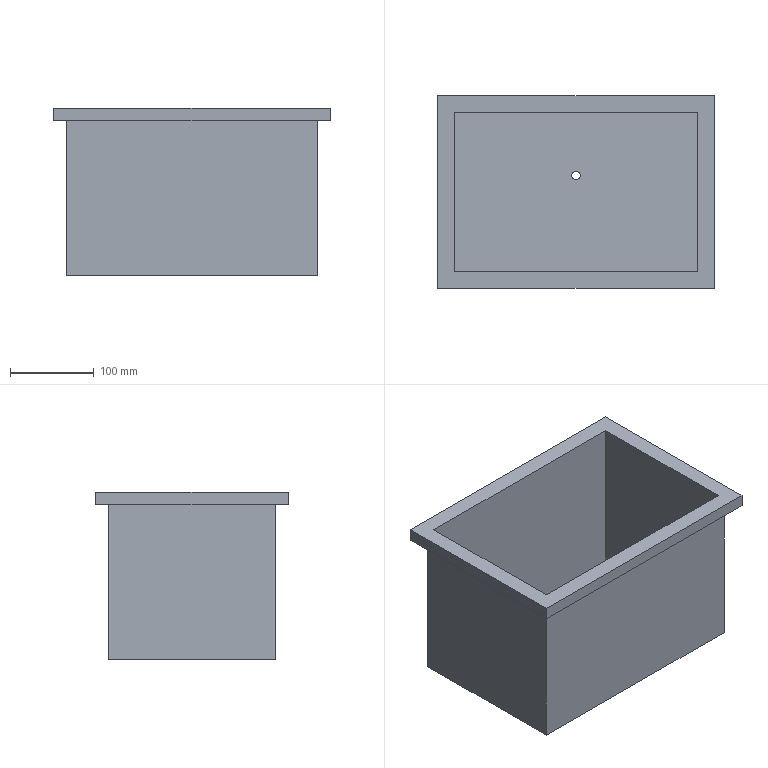Part | STEP file | Material box - copy | 1 solid | 18 faces | box 330 x 230 x 200 mm | volume 1493607 mm3 | plane 16 | cylinder 2 | commonest cylinder face diameters 10 x2
STEP:
#1=CARTESIAN_POINT('',(0.,0.,0.));
#2=DIRECTION('',(0.,0.,1.));
#3=DIRECTION('',(1.,0.,0.));
#4=AXIS2_PLACEMENT_3D('',#1,#2,#3);
#5=CARTESIAN_POINT('',(5.,20.,0.));
#6=VERTEX_POINT('',#5);
#7=CARTESIAN_POINT('',(5.,20.,5.));
#8=VERTEX_POINT('',#7);
#9=CARTESIAN_POINT('',(5.,20.,-5.));
#10=DIRECTION('',(0.,0.,1.));
#11=VECTOR('',#10,1.);
#12=LINE('',#9,#11);
#13=CARTESIAN_POINT('',(0.,20.,-5.));
#14=DIRECTION('',(0.,0.,1.));
#15=DIRECTION('',(1.,0.,0.));
#16=AXIS2_PLACEMENT_3D('',#13,#14,#15);
#17=CYLINDRICAL_SURFACE('',#16,5.);
#18=CARTESIAN_POINT('',(6.283,0.));
#19=DIRECTION('',(0.,1.));
#20=VECTOR('',#19,1.);
#21=LINE('',#18,#20);
#22=(GEOMETRIC_REPRESENTATION_CONTEXT(2)PARAMETRIC_REPRESENTATION_CONTEXT()REPRESENTATION_CONTEXT('',''));
#23=DEFINITIONAL_REPRESENTATION('',(#21),#22);
#24=PCURVE('',#17,#23);
#25=CARTESIAN_POINT('',(0.,20.,-5.));
#26=DIRECTION('',(0.,0.,1.));
#27=DIRECTION('',(1.,0.,0.));
#28=AXIS2_PLACEMENT_3D('',#25,#26,#27);
#29=CYLINDRICAL_SURFACE('',#28,5.);
#30=CARTESIAN_POINT('',(0.,0.));
#31=DIRECTION('',(0.,1.));
#32=VECTOR('',#31,1.);
#33=LINE('',#30,#32);
#34=(GEOMETRIC_REPRESENTATION_CONTEXT(2)PARAMETRIC_REPRESENTATION_CONTEXT()REPRESENTATION_CONTEXT('',''));
#35=DEFINITIONAL_REPRESENTATION('',(#33),#34);
#36=PCURVE('',#29,#35);
#37=SURFACE_CURVE('',#12,(#24,#36),.PCURVE_S1.);
#38=EDGE_CURVE('',#6,#8,#37,.T.);
#39=ORIENTED_EDGE('',*,*,#38,.T.);
#40=CARTESIAN_POINT('',(-5.,20.,5.));
#41=VERTEX_POINT('',#40);
#42=CARTESIAN_POINT('',(0.,20.,5.));
#43=DIRECTION('',(0.,0.,-1.));
#44=DIRECTION('',(1.,0.,0.));
#45=AXIS2_PLACEMENT_3D('',#42,#43,#44);
#46=CIRCLE('',#45,5.);
#47=CARTESIAN_POINT('',(6.283,10.));
#48=DIRECTION('',(-1.,0.));
#49=VECTOR('',#48,1.);
#50=LINE('',#47,#49);
#51=(GEOMETRIC_REPRESENTATION_CONTEXT(2)PARAMETRIC_REPRESENTATION_CONTEXT()REPRESENTATION_CONTEXT('',''));
#52=DEFINITIONAL_REPRESENTATION('',(#50),#51);
#53=PCURVE('',#17,#52);
#54=CARTESIAN_POINT('',(0.,0.,5.));
#55=DIRECTION('',(0.,0.,1.));
#56=DIRECTION('',(1.,0.,0.));
#57=AXIS2_PLACEMENT_3D('',#54,#55,#56);
#58=PLANE('',#57);
#59=CARTESIAN_POINT('',(5.,20.));
#60=CARTESIAN_POINT('',(5.,11.34));
#61=CARTESIAN_POINT('',(-2.5,15.67));
#62=CARTESIAN_POINT('',(-10.,20.));
#63=CARTESIAN_POINT('',(-2.5,24.33));
#64=CARTESIAN_POINT('',(5.,28.66));
#65=CARTESIAN_POINT('',(5.,20.));
#66=(BOUNDED_CURVE()B_SPLINE_CURVE(2,(#59,#60,#61,#62,#63,#64,#65),.UNSPECIFIED.,.T.,.F.)B_SPLINE_CURVE_WITH_KNOTS((1,2,2,2,2,1),(-2.094,0.,2.094,4.189,6.283,8.378),.UNSPECIFIED.)CURVE()GEOMETRIC_REPRESENTATION_ITEM()RATIONAL_B_SPLINE_CURVE((1.,0.5,1.,0.5,1.,0.5,1.))REPRESENTATION_ITEM(''));
#67=(GEOMETRIC_REPRESENTATION_CONTEXT(2)PARAMETRIC_REPRESENTATION_CONTEXT()REPRESENTATION_CONTEXT('',''));
#68=DEFINITIONAL_REPRESENTATION('',(#66),#67);
#69=PCURVE('',#58,#68);
#70=SURFACE_CURVE('',#46,(#53,#69),.PCURVE_S1.);
#71=EDGE_CURVE('',#8,#41,#70,.T.);
#72=ORIENTED_EDGE('',*,*,#71,.T.);
#73=CARTESIAN_POINT('',(-5.,20.,0.));
#74=VERTEX_POINT('',#73);
#75=CARTESIAN_POINT('',(-5.,20.,-5.));
#76=DIRECTION('',(0.,0.,1.));
#77=VECTOR('',#76,1.);
#78=LINE('',#75,#77);
#79=CARTESIAN_POINT('',(3.142,0.));
#80=DIRECTION('',(0.,1.));
#81=VECTOR('',#80,1.);
#82=LINE('',#79,#81);
#83=(GEOMETRIC_REPRESENTATION_CONTEXT(2)PARAMETRIC_REPRESENTATION_CONTEXT()REPRESENTATION_CONTEXT('',''));
#84=DEFINITIONAL_REPRESENTATION('',(#82),#83);
#85=PCURVE('',#17,#84);
#86=CARTESIAN_POINT('',(3.142,0.));
#87=DIRECTION('',(0.,1.));
#88=VECTOR('',#87,1.);
#89=LINE('',#86,#88);
#90=(GEOMETRIC_REPRESENTATION_CONTEXT(2)PARAMETRIC_REPRESENTATION_CONTEXT()REPRESENTATION_CONTEXT('',''));
#91=DEFINITIONAL_REPRESENTATION('',(#89),#90);
#92=PCURVE('',#29,#91);
#93=SURFACE_CURVE('',#78,(#85,#92),.PCURVE_S1.);
#94=EDGE_CURVE('',#74,#41,#93,.T.);
#95=ORIENTED_EDGE('',*,*,#94,.F.);
#96=CARTESIAN_POINT('',(0.,20.,0.));
#97=DIRECTION('',(0.,0.,-1.));
#98=DIRECTION('',(1.,0.,0.));
#99=AXIS2_PLACEMENT_3D('',#96,#97,#98);
#100=CIRCLE('',#99,5.);
#101=CARTESIAN_POINT('',(6.283,5.));
#102=DIRECTION('',(-1.,0.));
#103=VECTOR('',#102,1.);
#104=LINE('',#101,#103);
#105=(GEOMETRIC_REPRESENTATION_CONTEXT(2)PARAMETRIC_REPRESENTATION_CONTEXT()REPRESENTATION_CONTEXT('',''));
#106=DEFINITIONAL_REPRESENTATION('',(#104),#105);
#107=PCURVE('',#17,#106);
#108=CARTESIAN_POINT('',(0.,0.,0.));
#109=DIRECTION('',(0.,0.,1.));
#110=DIRECTION('',(1.,0.,0.));
#111=AXIS2_PLACEMENT_3D('',#108,#109,#110);
#112=PLANE('',#111);
#113=CARTESIAN_POINT('',(5.,20.));
#114=CARTESIAN_POINT('',(5.,11.34));
#115=CARTESIAN_POINT('',(-2.5,15.67));
#116=CARTESIAN_POINT('',(-10.,20.));
#117=CARTESIAN_POINT('',(-2.5,24.33));
#118=CARTESIAN_POINT('',(5.,28.66));
#119=CARTESIAN_POINT('',(5.,20.));
#120=(BOUNDED_CURVE()B_SPLINE_CURVE(2,(#113,#114,#115,#116,#117,#118,#119),.UNSPECIFIED.,.T.,.F.)B_SPLINE_CURVE_WITH_KNOTS((1,2,2,2,2,1),(-2.094,0.,2.094,4.189,6.283,8.378),.UNSPECIFIED.)CURVE()GEOMETRIC_REPRESENTATION_ITEM()RATIONAL_B_SPLINE_CURVE((1.,0.5,1.,0.5,1.,0.5,1.))REPRESENTATION_ITEM(''));
#121=(GEOMETRIC_REPRESENTATION_CONTEXT(2)PARAMETRIC_REPRESENTATION_CONTEXT()REPRESENTATION_CONTEXT('',''));
#122=DEFINITIONAL_REPRESENTATION('',(#120),#121);
#123=PCURVE('',#112,#122);
#124=SURFACE_CURVE('',#100,(#107,#123),.PCURVE_S1.);
#125=EDGE_CURVE('',#6,#74,#124,.T.);
#126=ORIENTED_EDGE('',*,*,#125,.F.);
#127=EDGE_LOOP('',(#39,#72,#95,#126));
#128=FACE_BOUND('',#127,.F.);
#129=ADVANCED_FACE('',(#128),#17,.F.);
#130=CARTESIAN_POINT('',(-150.,-100.,0.));
#131=VERTEX_POINT('',#130);
#132=CARTESIAN_POINT('',(150.,-100.,0.));
#133=VERTEX_POINT('',#132);
#134=CARTESIAN_POINT('',(0.,-100.,0.));
#135=DIRECTION('',(1.,0.,0.));
#136=VECTOR('',#135,1.);
#137=LINE('',#134,#136);
#138=CARTESIAN_POINT('',(0.,-100.));
#139=DIRECTION('',(1.,0.));
#140=VECTOR('',#139,1.);
#141=LINE('',#138,#140);
#142=(GEOMETRIC_REPRESENTATION_CONTEXT(2)PARAMETRIC_REPRESENTATION_CONTEXT()REPRESENTATION_CONTEXT('',''));
#143=DEFINITIONAL_REPRESENTATION('',(#141),#142);
#144=PCURVE('',#112,#143);
#145=CARTESIAN_POINT('',(-150.,-100.,200.));
#146=DIRECTION('',(0.,1.,0.));
#147=DIRECTION('',(0.,0.,1.));
#148=AXIS2_PLACEMENT_3D('',#145,#146,#147);
#149=PLANE('',#148);
#150=CARTESIAN_POINT('',(-200.,150.));
#151=DIRECTION('',(0.,1.));
#152=VECTOR('',#151,1.);
#153=LINE('',#150,#152);
#154=(GEOMETRIC_REPRESENTATION_CONTEXT(2)PARAMETRIC_REPRESENTATION_CONTEXT()REPRESENTATION_CONTEXT('',''));
#155=DEFINITIONAL_REPRESENTATION('',(#153),#154);
#156=PCURVE('',#149,#155);
#157=SURFACE_CURVE('',#137,(#144,#156),.PCURVE_S1.);
#158=EDGE_CURVE('',#131,#133,#157,.T.);
#159=ORIENTED_EDGE('',*,*,#158,.F.);
#160=CARTESIAN_POINT('',(-150.,100.,0.));
#161=VERTEX_POINT('',#160);
#162=CARTESIAN_POINT('',(-150.,0.,0.));
#163=DIRECTION('',(0.,-1.,0.));
#164=VECTOR('',#163,1.);
#165=LINE('',#162,#164);
#166=CARTESIAN_POINT('',(-150.,0.));
#167=DIRECTION('',(0.,-1.));
#168=VECTOR('',#167,1.);
#169=LINE('',#166,#168);
#170=(GEOMETRIC_REPRESENTATION_CONTEXT(2)PARAMETRIC_REPRESENTATION_CONTEXT()REPRESENTATION_CONTEXT('',''));
#171=DEFINITIONAL_REPRESENTATION('',(#169),#170);
#172=PCURVE('',#112,#171);
#173=CARTESIAN_POINT('',(-150.,100.,200.));
#174=DIRECTION('',(1.,0.,0.));
#175=DIRECTION('',(0.,0.,-1.));
#176=AXIS2_PLACEMENT_3D('',#173,#174,#175);
#177=PLANE('',#176);
#178=CARTESIAN_POINT('',(200.,-100.));
#179=DIRECTION('',(0.,-1.));
#180=VECTOR('',#179,1.);
#181=LINE('',#178,#180);
#182=(GEOMETRIC_REPRESENTATION_CONTEXT(2)PARAMETRIC_REPRESENTATION_CONTEXT()REPRESENTATION_CONTEXT('',''));
#183=DEFINITIONAL_REPRESENTATION('',(#181),#182);
#184=PCURVE('',#177,#183);
#185=SURFACE_CURVE('',#165,(#172,#184),.PCURVE_S1.);
#186=EDGE_CURVE('',#161,#131,#185,.T.);
#187=ORIENTED_EDGE('',*,*,#186,.F.);
#188=CARTESIAN_POINT('',(150.,100.,0.));
#189=VERTEX_POINT('',#188);
#190=CARTESIAN_POINT('',(0.,100.,0.));
#191=DIRECTION('',(-1.,0.,0.));
#192=VECTOR('',#191,1.);
#193=LINE('',#190,#192);
#194=CARTESIAN_POINT('',(0.,100.));
#195=DIRECTION('',(-1.,0.));
#196=VECTOR('',#195,1.);
#197=LINE('',#194,#196);
#198=(GEOMETRIC_REPRESENTATION_CONTEXT(2)PARAMETRIC_REPRESENTATION_CONTEXT()REPRESENTATION_CONTEXT('',''));
#199=DEFINITIONAL_REPRESENTATION('',(#197),#198);
#200=PCURVE('',#112,#199);
#201=CARTESIAN_POINT('',(-150.,100.,200.));
#202=DIRECTION('',(0.,-1.,0.));
#203=DIRECTION('',(0.,0.,-1.));
#204=AXIS2_PLACEMENT_3D('',#201,#202,#203);
#205=PLANE('',#204);
#206=CARTESIAN_POINT('',(200.,150.));
#207=DIRECTION('',(0.,-1.));
#208=VECTOR('',#207,1.);
#209=LINE('',#206,#208);
#210=(GEOMETRIC_REPRESENTATION_CONTEXT(2)PARAMETRIC_REPRESENTATION_CONTEXT()REPRESENTATION_CONTEXT('',''));
#211=DEFINITIONAL_REPRESENTATION('',(#209),#210);
#212=PCURVE('',#205,#211);
#213=SURFACE_CURVE('',#193,(#200,#212),.PCURVE_S1.);
#214=EDGE_CURVE('',#189,#161,#213,.T.);
#215=ORIENTED_EDGE('',*,*,#214,.F.);
#216=CARTESIAN_POINT('',(150.,0.,0.));
#217=DIRECTION('',(0.,1.,0.));
#218=VECTOR('',#217,1.);
#219=LINE('',#216,#218);
#220=CARTESIAN_POINT('',(150.,0.));
#221=DIRECTION('',(0.,1.));
#222=VECTOR('',#221,1.);
#223=LINE('',#220,#222);
#224=(GEOMETRIC_REPRESENTATION_CONTEXT(2)PARAMETRIC_REPRESENTATION_CONTEXT()REPRESENTATION_CONTEXT('',''));
#225=DEFINITIONAL_REPRESENTATION('',(#223),#224);
#226=PCURVE('',#112,#225);
#227=CARTESIAN_POINT('',(150.,100.,200.));
#228=DIRECTION('',(-1.,0.,0.));
#229=DIRECTION('',(0.,0.,1.));
#230=AXIS2_PLACEMENT_3D('',#227,#228,#229);
#231=PLANE('',#230);
#232=CARTESIAN_POINT('',(-200.,-100.));
#233=DIRECTION('',(0.,1.));
#234=VECTOR('',#233,1.);
#235=LINE('',#232,#234);
#236=(GEOMETRIC_REPRESENTATION_CONTEXT(2)PARAMETRIC_REPRESENTATION_CONTEXT()REPRESENTATION_CONTEXT('',''));
#237=DEFINITIONAL_REPRESENTATION('',(#235),#236);
#238=PCURVE('',#231,#237);
#239=SURFACE_CURVE('',#219,(#226,#238),.PCURVE_S1.);
#240=EDGE_CURVE('',#133,#189,#239,.T.);
#241=ORIENTED_EDGE('',*,*,#240,.F.);
#242=EDGE_LOOP('',(#159,#187,#215,#241));
#243=FACE_BOUND('',#242,.T.);
#244=ORIENTED_EDGE('',*,*,#125,.F.);
#245=CARTESIAN_POINT('',(0.,20.,0.));
#246=DIRECTION('',(0.,0.,-1.));
#247=DIRECTION('',(1.,0.,0.));
#248=AXIS2_PLACEMENT_3D('',#245,#246,#247);
#249=CIRCLE('',#248,5.);
#250=CARTESIAN_POINT('',(5.,20.));
#251=CARTESIAN_POINT('',(5.,11.34));
#252=CARTESIAN_POINT('',(-2.5,15.67));
#253=CARTESIAN_POINT('',(-10.,20.));
#254=CARTESIAN_POINT('',(-2.5,24.33));
#255=CARTESIAN_POINT('',(5.,28.66));
#256=CARTESIAN_POINT('',(5.,20.));
#257=(BOUNDED_CURVE()B_SPLINE_CURVE(2,(#250,#251,#252,#253,#254,#255,#256),.UNSPECIFIED.,.T.,.F.)B_SPLINE_CURVE_WITH_KNOTS((1,2,2,2,2,1),(-2.094,0.,2.094,4.189,6.283,8.378),.UNSPECIFIED.)CURVE()GEOMETRIC_REPRESENTATION_ITEM()RATIONAL_B_SPLINE_CURVE((1.,0.5,1.,0.5,1.,0.5,1.))REPRESENTATION_ITEM(''));
#258=(GEOMETRIC_REPRESENTATION_CONTEXT(2)PARAMETRIC_REPRESENTATION_CONTEXT()REPRESENTATION_CONTEXT('',''));
#259=DEFINITIONAL_REPRESENTATION('',(#257),#258);
#260=PCURVE('',#112,#259);
#261=CARTESIAN_POINT('',(6.283,5.));
#262=DIRECTION('',(-1.,0.));
#263=VECTOR('',#262,1.);
#264=LINE('',#261,#263);
#265=(GEOMETRIC_REPRESENTATION_CONTEXT(2)PARAMETRIC_REPRESENTATION_CONTEXT()REPRESENTATION_CONTEXT('',''));
#266=DEFINITIONAL_REPRESENTATION('',(#264),#265);
#267=PCURVE('',#29,#266);
#268=SURFACE_CURVE('',#249,(#260,#267),.PCURVE_S1.);
#269=EDGE_CURVE('',#74,#6,#268,.T.);
#270=ORIENTED_EDGE('',*,*,#269,.F.);
#271=EDGE_LOOP('',(#244,#270));
#272=FACE_BOUND('',#271,.T.);
#273=ADVANCED_FACE('',(#243,#272),#112,.F.);
#274=CARTESIAN_POINT('',(150.,-100.,185.));
#275=VERTEX_POINT('',#274);
#276=CARTESIAN_POINT('',(150.,100.,185.));
#277=VERTEX_POINT('',#276);
#278=CARTESIAN_POINT('',(150.,100.,185.));
#279=DIRECTION('',(0.,1.,0.));
#280=VECTOR('',#279,1.);
#281=LINE('',#278,#280);
#282=CARTESIAN_POINT('',(-15.,0.));
#283=DIRECTION('',(0.,1.));
#284=VECTOR('',#283,1.);
#285=LINE('',#282,#284);
#286=(GEOMETRIC_REPRESENTATION_CONTEXT(2)PARAMETRIC_REPRESENTATION_CONTEXT()REPRESENTATION_CONTEXT('',''));
#287=DEFINITIONAL_REPRESENTATION('',(#285),#286);
#288=PCURVE('',#231,#287);
#289=CARTESIAN_POINT('',(0.,0.,185.));
#290=DIRECTION('',(0.,0.,-1.));
#291=DIRECTION('',(-1.,0.,0.));
#292=AXIS2_PLACEMENT_3D('',#289,#290,#291);
#293=PLANE('',#292);
#294=CARTESIAN_POINT('',(-150.,100.));
#295=DIRECTION('',(0.,1.));
#296=VECTOR('',#295,1.);
#297=LINE('',#294,#296);
#298=(GEOMETRIC_REPRESENTATION_CONTEXT(2)PARAMETRIC_REPRESENTATION_CONTEXT()REPRESENTATION_CONTEXT('',''));
#299=DEFINITIONAL_REPRESENTATION('',(#297),#298);
#300=PCURVE('',#293,#299);
#301=SURFACE_CURVE('',#281,(#288,#300),.PCURVE_S1.);
#302=EDGE_CURVE('',#275,#277,#301,.T.);
#303=ORIENTED_EDGE('',*,*,#302,.F.);
#304=CARTESIAN_POINT('',(150.,-100.,200.));
#305=DIRECTION('',(0.,0.,1.));
#306=VECTOR('',#305,1.);
#307=LINE('',#304,#306);
#308=CARTESIAN_POINT('',(0.,-200.));
#309=DIRECTION('',(1.,0.));
#310=VECTOR('',#309,1.);
#311=LINE('',#308,#310);
#312=(GEOMETRIC_REPRESENTATION_CONTEXT(2)PARAMETRIC_REPRESENTATION_CONTEXT()REPRESENTATION_CONTEXT('',''));
#313=DEFINITIONAL_REPRESENTATION('',(#311),#312);
#314=PCURVE('',#231,#313);
#315=CARTESIAN_POINT('',(0.,300.));
#316=DIRECTION('',(1.,0.));
#317=VECTOR('',#316,1.);
#318=LINE('',#315,#317);
#319=(GEOMETRIC_REPRESENTATION_CONTEXT(2)PARAMETRIC_REPRESENTATION_CONTEXT()REPRESENTATION_CONTEXT('',''));
#320=DEFINITIONAL_REPRESENTATION('',(#318),#319);
#321=PCURVE('',#149,#320);
#322=SURFACE_CURVE('',#307,(#314,#321),.PCURVE_S1.);
#323=EDGE_CURVE('',#133,#275,#322,.T.);
#324=ORIENTED_EDGE('',*,*,#323,.F.);
#325=ORIENTED_EDGE('',*,*,#240,.T.);
#326=CARTESIAN_POINT('',(150.,100.,200.));
#327=DIRECTION('',(0.,0.,-1.));
#328=VECTOR('',#327,1.);
#329=LINE('',#326,#328);
#330=CARTESIAN_POINT('',(0.,0.));
#331=DIRECTION('',(-1.,0.));
#332=VECTOR('',#331,1.);
#333=LINE('',#330,#332);
#334=(GEOMETRIC_REPRESENTATION_CONTEXT(2)PARAMETRIC_REPRESENTATION_CONTEXT()REPRESENTATION_CONTEXT('',''));
#335=DEFINITIONAL_REPRESENTATION('',(#333),#334);
#336=PCURVE('',#231,#335);
#337=CARTESIAN_POINT('',(0.,300.));
#338=DIRECTION('',(1.,0.));
#339=VECTOR('',#338,1.);
#340=LINE('',#337,#339);
#341=(GEOMETRIC_REPRESENTATION_CONTEXT(2)PARAMETRIC_REPRESENTATION_CONTEXT()REPRESENTATION_CONTEXT('',''));
#342=DEFINITIONAL_REPRESENTATION('',(#340),#341);
#343=PCURVE('',#205,#342);
#344=SURFACE_CURVE('',#329,(#336,#343),.PCURVE_S1.);
#345=EDGE_CURVE('',#277,#189,#344,.T.);
#346=ORIENTED_EDGE('',*,*,#345,.F.);
#347=EDGE_LOOP('',(#303,#324,#325,#346));
#348=FACE_BOUND('',#347,.T.);
#349=ADVANCED_FACE('',(#348),#231,.F.);
#350=CARTESIAN_POINT('',(-150.,-100.,185.));
#351=VERTEX_POINT('',#350);
#352=CARTESIAN_POINT('',(-150.,-100.,185.));
#353=DIRECTION('',(1.,0.,0.));
#354=VECTOR('',#353,1.);
#355=LINE('',#352,#354);
#356=CARTESIAN_POINT('',(-15.,0.));
#357=DIRECTION('',(0.,1.));
#358=VECTOR('',#357,1.);
#359=LINE('',#356,#358);
#360=(GEOMETRIC_REPRESENTATION_CONTEXT(2)PARAMETRIC_REPRESENTATION_CONTEXT()REPRESENTATION_CONTEXT('',''));
#361=DEFINITIONAL_REPRESENTATION('',(#359),#360);
#362=PCURVE('',#149,#361);
#363=CARTESIAN_POINT('',(150.,-100.));
#364=DIRECTION('',(-1.,0.));
#365=VECTOR('',#364,1.);
#366=LINE('',#363,#365);
#367=(GEOMETRIC_REPRESENTATION_CONTEXT(2)PARAMETRIC_REPRESENTATION_CONTEXT()REPRESENTATION_CONTEXT('',''));
#368=DEFINITIONAL_REPRESENTATION('',(#366),#367);
#369=PCURVE('',#293,#368);
#370=SURFACE_CURVE('',#355,(#362,#369),.PCURVE_S1.);
#371=EDGE_CURVE('',#351,#275,#370,.T.);
#372=ORIENTED_EDGE('',*,*,#371,.F.);
#373=CARTESIAN_POINT('',(-150.,-100.,200.));
#374=DIRECTION('',(0.,0.,1.));
#375=VECTOR('',#374,1.);
#376=LINE('',#373,#375);
#377=CARTESIAN_POINT('',(0.,0.));
#378=DIRECTION('',(1.,0.));
#379=VECTOR('',#378,1.);
#380=LINE('',#377,#379);
#381=(GEOMETRIC_REPRESENTATION_CONTEXT(2)PARAMETRIC_REPRESENTATION_CONTEXT()REPRESENTATION_CONTEXT('',''));
#382=DEFINITIONAL_REPRESENTATION('',(#380),#381);
#383=PCURVE('',#149,#382);
#384=CARTESIAN_POINT('',(0.,-200.));
#385=DIRECTION('',(-1.,0.));
#386=VECTOR('',#385,1.);
#387=LINE('',#384,#386);
#388=(GEOMETRIC_REPRESENTATION_CONTEXT(2)PARAMETRIC_REPRESENTATION_CONTEXT()REPRESENTATION_CONTEXT('',''));
#389=DEFINITIONAL_REPRESENTATION('',(#387),#388);
#390=PCURVE('',#177,#389);
#391=SURFACE_CURVE('',#376,(#383,#390),.PCURVE_S1.);
#392=EDGE_CURVE('',#131,#351,#391,.T.);
#393=ORIENTED_EDGE('',*,*,#392,.F.);
#394=ORIENTED_EDGE('',*,*,#158,.T.);
#395=ORIENTED_EDGE('',*,*,#323,.T.);
#396=EDGE_LOOP('',(#372,#393,#394,#395));
#397=FACE_BOUND('',#396,.T.);
#398=ADVANCED_FACE('',(#397),#149,.F.);
#399=CARTESIAN_POINT('',(-150.,100.,185.));
#400=VERTEX_POINT('',#399);
#401=CARTESIAN_POINT('',(-150.,100.,185.));
#402=DIRECTION('',(0.,-1.,0.));
#403=VECTOR('',#402,1.);
#404=LINE('',#401,#403);
#405=CARTESIAN_POINT('',(15.,0.));
#406=DIRECTION('',(0.,-1.));
#407=VECTOR('',#406,1.);
#408=LINE('',#405,#407);
#409=(GEOMETRIC_REPRESENTATION_CONTEXT(2)PARAMETRIC_REPRESENTATION_CONTEXT()REPRESENTATION_CONTEXT('',''));
#410=DEFINITIONAL_REPRESENTATION('',(#408),#409);
#411=PCURVE('',#177,#410);
#412=CARTESIAN_POINT('',(150.,100.));
#413=DIRECTION('',(0.,-1.));
#414=VECTOR('',#413,1.);
#415=LINE('',#412,#414);
#416=(GEOMETRIC_REPRESENTATION_CONTEXT(2)PARAMETRIC_REPRESENTATION_CONTEXT()REPRESENTATION_CONTEXT('',''));
#417=DEFINITIONAL_REPRESENTATION('',(#415),#416);
#418=PCURVE('',#293,#417);
#419=SURFACE_CURVE('',#404,(#411,#418),.PCURVE_S1.);
#420=EDGE_CURVE('',#400,#351,#419,.T.);
#421=ORIENTED_EDGE('',*,*,#420,.F.);
#422=CARTESIAN_POINT('',(-150.,100.,200.));
#423=DIRECTION('',(0.,0.,1.));
#424=VECTOR('',#423,1.);
#425=LINE('',#422,#424);
#426=CARTESIAN_POINT('',(0.,0.));
#427=DIRECTION('',(-1.,0.));
#428=VECTOR('',#427,1.);
#429=LINE('',#426,#428);
#430=(GEOMETRIC_REPRESENTATION_CONTEXT(2)PARAMETRIC_REPRESENTATION_CONTEXT()REPRESENTATION_CONTEXT('',''));
#431=DEFINITIONAL_REPRESENTATION('',(#429),#430);
#432=PCURVE('',#177,#431);
#433=CARTESIAN_POINT('',(0.,0.));
#434=DIRECTION('',(-1.,0.));
#435=VECTOR('',#434,1.);
#436=LINE('',#433,#435);
#437=(GEOMETRIC_REPRESENTATION_CONTEXT(2)PARAMETRIC_REPRESENTATION_CONTEXT()REPRESENTATION_CONTEXT('',''));
#438=DEFINITIONAL_REPRESENTATION('',(#436),#437);
#439=PCURVE('',#205,#438);
#440=SURFACE_CURVE('',#425,(#432,#439),.PCURVE_S1.);
#441=EDGE_CURVE('',#161,#400,#440,.T.);
#442=ORIENTED_EDGE('',*,*,#441,.F.);
#443=ORIENTED_EDGE('',*,*,#186,.T.);
#444=ORIENTED_EDGE('',*,*,#392,.T.);
#445=EDGE_LOOP('',(#421,#442,#443,#444));
#446=FACE_BOUND('',#445,.T.);
#447=ADVANCED_FACE('',(#446),#177,.F.);
#448=CARTESIAN_POINT('',(-150.,100.,185.));
#449=DIRECTION('',(-1.,0.,0.));
#450=VECTOR('',#449,1.);
#451=LINE('',#448,#450);
#452=CARTESIAN_POINT('',(15.,0.));
#453=DIRECTION('',(0.,-1.));
#454=VECTOR('',#453,1.);
#455=LINE('',#452,#454);
#456=(GEOMETRIC_REPRESENTATION_CONTEXT(2)PARAMETRIC_REPRESENTATION_CONTEXT()REPRESENTATION_CONTEXT('',''));
#457=DEFINITIONAL_REPRESENTATION('',(#455),#456);
#458=PCURVE('',#205,#457);
#459=CARTESIAN_POINT('',(150.,100.));
#460=DIRECTION('',(1.,0.));
#461=VECTOR('',#460,1.);
#462=LINE('',#459,#461);
#463=(GEOMETRIC_REPRESENTATION_CONTEXT(2)PARAMETRIC_REPRESENTATION_CONTEXT()REPRESENTATION_CONTEXT('',''));
#464=DEFINITIONAL_REPRESENTATION('',(#462),#463);
#465=PCURVE('',#293,#464);
#466=SURFACE_CURVE('',#451,(#458,#465),.PCURVE_S1.);
#467=EDGE_CURVE('',#277,#400,#466,.T.);
#468=ORIENTED_EDGE('',*,*,#467,.F.);
#469=ORIENTED_EDGE('',*,*,#345,.T.);
#470=ORIENTED_EDGE('',*,*,#214,.T.);
#471=ORIENTED_EDGE('',*,*,#441,.T.);
#472=EDGE_LOOP('',(#468,#469,#470,#471));
#473=FACE_BOUND('',#472,.T.);
#474=ADVANCED_FACE('',(#473),#205,.F.);
#475=CARTESIAN_POINT('',(0.,20.,5.));
#476=DIRECTION('',(0.,0.,-1.));
#477=DIRECTION('',(1.,0.,0.));
#478=AXIS2_PLACEMENT_3D('',#475,#476,#477);
#479=CIRCLE('',#478,5.);
#480=CARTESIAN_POINT('',(6.283,10.));
#481=DIRECTION('',(-1.,0.));
#482=VECTOR('',#481,1.);
#483=LINE('',#480,#482);
#484=(GEOMETRIC_REPRESENTATION_CONTEXT(2)PARAMETRIC_REPRESENTATION_CONTEXT()REPRESENTATION_CONTEXT('',''));
#485=DEFINITIONAL_REPRESENTATION('',(#483),#484);
#486=PCURVE('',#29,#485);
#487=CARTESIAN_POINT('',(5.,20.));
#488=CARTESIAN_POINT('',(5.,11.34));
#489=CARTESIAN_POINT('',(-2.5,15.67));
#490=CARTESIAN_POINT('',(-10.,20.));
#491=CARTESIAN_POINT('',(-2.5,24.33));
#492=CARTESIAN_POINT('',(5.,28.66));
#493=CARTESIAN_POINT('',(5.,20.));
#494=(BOUNDED_CURVE()B_SPLINE_CURVE(2,(#487,#488,#489,#490,#491,#492,#493),.UNSPECIFIED.,.T.,.F.)B_SPLINE_CURVE_WITH_KNOTS((1,2,2,2,2,1),(-2.094,0.,2.094,4.189,6.283,8.378),.UNSPECIFIED.)CURVE()GEOMETRIC_REPRESENTATION_ITEM()RATIONAL_B_SPLINE_CURVE((1.,0.5,1.,0.5,1.,0.5,1.))REPRESENTATION_ITEM(''));
#495=(GEOMETRIC_REPRESENTATION_CONTEXT(2)PARAMETRIC_REPRESENTATION_CONTEXT()REPRESENTATION_CONTEXT('',''));
#496=DEFINITIONAL_REPRESENTATION('',(#494),#495);
#497=PCURVE('',#58,#496);
#498=SURFACE_CURVE('',#479,(#486,#497),.PCURVE_S1.);
#499=EDGE_CURVE('',#41,#8,#498,.T.);
#500=ORIENTED_EDGE('',*,*,#499,.T.);
#501=ORIENTED_EDGE('',*,*,#38,.F.);
#502=ORIENTED_EDGE('',*,*,#269,.F.);
#503=ORIENTED_EDGE('',*,*,#94,.T.);
#504=EDGE_LOOP('',(#500,#501,#502,#503));
#505=FACE_BOUND('',#504,.F.);
#506=ADVANCED_FACE('',(#505),#29,.F.);
#507=CARTESIAN_POINT('',(165.,-115.,185.));
#508=VERTEX_POINT('',#507);
#509=CARTESIAN_POINT('',(-165.,-115.,185.));
#510=VERTEX_POINT('',#509);
#511=CARTESIAN_POINT('',(0.,-115.,185.));
#512=DIRECTION('',(-1.,0.,0.));
#513=VECTOR('',#512,1.);
#514=LINE('',#511,#513);
#515=CARTESIAN_POINT('',(0.,-115.));
#516=DIRECTION('',(1.,0.));
#517=VECTOR('',#516,1.);
#518=LINE('',#515,#517);
#519=(GEOMETRIC_REPRESENTATION_CONTEXT(2)PARAMETRIC_REPRESENTATION_CONTEXT()REPRESENTATION_CONTEXT('',''));
#520=DEFINITIONAL_REPRESENTATION('',(#518),#519);
#521=PCURVE('',#293,#520);
#522=CARTESIAN_POINT('',(-165.,-115.,185.));
#523=DIRECTION('',(0.,-1.,0.));
#524=DIRECTION('',(1.,0.,0.));
#525=AXIS2_PLACEMENT_3D('',#522,#523,#524);
#526=PLANE('',#525);
#527=CARTESIAN_POINT('',(165.,0.));
#528=DIRECTION('',(-1.,0.));
#529=VECTOR('',#528,1.);
#530=LINE('',#527,#529);
#531=(GEOMETRIC_REPRESENTATION_CONTEXT(2)PARAMETRIC_REPRESENTATION_CONTEXT()REPRESENTATION_CONTEXT('',''));
#532=DEFINITIONAL_REPRESENTATION('',(#530),#531);
#533=PCURVE('',#526,#532);
#534=SURFACE_CURVE('',#514,(#521,#533),.PCURVE_S1.);
#535=EDGE_CURVE('',#508,#510,#534,.T.);
#536=ORIENTED_EDGE('',*,*,#535,.T.);
#537=CARTESIAN_POINT('',(-165.,115.,185.));
#538=VERTEX_POINT('',#537);
#539=CARTESIAN_POINT('',(-165.,0.,185.));
#540=DIRECTION('',(0.,1.,0.));
#541=VECTOR('',#540,1.);
#542=LINE('',#539,#541);
#543=CARTESIAN_POINT('',(165.,0.));
#544=DIRECTION('',(0.,1.));
#545=VECTOR('',#544,1.);
#546=LINE('',#543,#545);
#547=(GEOMETRIC_REPRESENTATION_CONTEXT(2)PARAMETRIC_REPRESENTATION_CONTEXT()REPRESENTATION_CONTEXT('',''));
#548=DEFINITIONAL_REPRESENTATION('',(#546),#547);
#549=PCURVE('',#293,#548);
#550=CARTESIAN_POINT('',(-165.,115.,185.));
#551=DIRECTION('',(-1.,0.,0.));
#552=DIRECTION('',(0.,-1.,0.));
#553=AXIS2_PLACEMENT_3D('',#550,#551,#552);
#554=PLANE('',#553);
#555=CARTESIAN_POINT('',(115.,0.));
#556=DIRECTION('',(-1.,0.));
#557=VECTOR('',#556,1.);
#558=LINE('',#555,#557);
#559=(GEOMETRIC_REPRESENTATION_CONTEXT(2)PARAMETRIC_REPRESENTATION_CONTEXT()REPRESENTATION_CONTEXT('',''));
#560=DEFINITIONAL_REPRESENTATION('',(#558),#559);
#561=PCURVE('',#554,#560);
#562=SURFACE_CURVE('',#542,(#549,#561),.PCURVE_S1.);
#563=EDGE_CURVE('',#510,#538,#562,.T.);
#564=ORIENTED_EDGE('',*,*,#563,.T.);
#565=CARTESIAN_POINT('',(165.,115.,185.));
#566=VERTEX_POINT('',#565);
#567=CARTESIAN_POINT('',(0.,115.,185.));
#568=DIRECTION('',(1.,0.,0.));
#569=VECTOR('',#568,1.);
#570=LINE('',#567,#569);
#571=CARTESIAN_POINT('',(0.,115.));
#572=DIRECTION('',(-1.,0.));
#573=VECTOR('',#572,1.);
#574=LINE('',#571,#573);
#575=(GEOMETRIC_REPRESENTATION_CONTEXT(2)PARAMETRIC_REPRESENTATION_CONTEXT()REPRESENTATION_CONTEXT('',''));
#576=DEFINITIONAL_REPRESENTATION('',(#574),#575);
#577=PCURVE('',#293,#576);
#578=CARTESIAN_POINT('',(-165.,115.,185.));
#579=DIRECTION('',(0.,1.,0.));
#580=DIRECTION('',(0.,0.,1.));
#581=AXIS2_PLACEMENT_3D('',#578,#579,#580);
#582=PLANE('',#581);
#583=CARTESIAN_POINT('',(0.,165.));
#584=DIRECTION('',(0.,1.));
#585=VECTOR('',#584,1.);
#586=LINE('',#583,#585);
#587=(GEOMETRIC_REPRESENTATION_CONTEXT(2)PARAMETRIC_REPRESENTATION_CONTEXT()REPRESENTATION_CONTEXT('',''));
#588=DEFINITIONAL_REPRESENTATION('',(#586),#587);
#589=PCURVE('',#582,#588);
#590=SURFACE_CURVE('',#570,(#577,#589),.PCURVE_S1.);
#591=EDGE_CURVE('',#538,#566,#590,.T.);
#592=ORIENTED_EDGE('',*,*,#591,.T.);
#593=CARTESIAN_POINT('',(165.,0.,185.));
#594=DIRECTION('',(0.,-1.,0.));
#595=VECTOR('',#594,1.);
#596=LINE('',#593,#595);
#597=CARTESIAN_POINT('',(-165.,0.));
#598=DIRECTION('',(0.,-1.));
#599=VECTOR('',#598,1.);
#600=LINE('',#597,#599);
#601=(GEOMETRIC_REPRESENTATION_CONTEXT(2)PARAMETRIC_REPRESENTATION_CONTEXT()REPRESENTATION_CONTEXT('',''));
#602=DEFINITIONAL_REPRESENTATION('',(#600),#601);
#603=PCURVE('',#293,#602);
#604=CARTESIAN_POINT('',(165.,115.,185.));
#605=DIRECTION('',(1.,0.,0.));
#606=DIRECTION('',(0.,1.,0.));
#607=AXIS2_PLACEMENT_3D('',#604,#605,#606);
#608=PLANE('',#607);
#609=CARTESIAN_POINT('',(-115.,0.));
#610=DIRECTION('',(-1.,0.));
#611=VECTOR('',#610,1.);
#612=LINE('',#609,#611);
#613=(GEOMETRIC_REPRESENTATION_CONTEXT(2)PARAMETRIC_REPRESENTATION_CONTEXT()REPRESENTATION_CONTEXT('',''));
#614=DEFINITIONAL_REPRESENTATION('',(#612),#613);
#615=PCURVE('',#608,#614);
#616=SURFACE_CURVE('',#596,(#603,#615),.PCURVE_S1.);
#617=EDGE_CURVE('',#566,#508,#616,.T.);
#618=ORIENTED_EDGE('',*,*,#617,.T.);
#619=EDGE_LOOP('',(#536,#564,#592,#618));
#620=FACE_BOUND('',#619,.T.);
#621=ORIENTED_EDGE('',*,*,#302,.T.);
#622=ORIENTED_EDGE('',*,*,#467,.T.);
#623=ORIENTED_EDGE('',*,*,#420,.T.);
#624=ORIENTED_EDGE('',*,*,#371,.T.);
#625=EDGE_LOOP('',(#621,#622,#623,#624));
#626=FACE_BOUND('',#625,.T.);
#627=ADVANCED_FACE('',(#620,#626),#293,.T.);
#628=CARTESIAN_POINT('',(-145.,95.,5.));
#629=VERTEX_POINT('',#628);
#630=CARTESIAN_POINT('',(-145.,-95.,5.));
#631=VERTEX_POINT('',#630);
#632=CARTESIAN_POINT('',(-145.,0.,5.));
#633=DIRECTION('',(0.,-1.,0.));
#634=VECTOR('',#633,1.);
#635=LINE('',#632,#634);
#636=CARTESIAN_POINT('',(-145.,0.));
#637=DIRECTION('',(0.,-1.));
#638=VECTOR('',#637,1.);
#639=LINE('',#636,#638);
#640=(GEOMETRIC_REPRESENTATION_CONTEXT(2)PARAMETRIC_REPRESENTATION_CONTEXT()REPRESENTATION_CONTEXT('',''));
#641=DEFINITIONAL_REPRESENTATION('',(#639),#640);
#642=PCURVE('',#58,#641);
#643=CARTESIAN_POINT('',(-145.,100.,200.));
#644=DIRECTION('',(1.,0.,0.));
#645=DIRECTION('',(0.,0.,-1.));
#646=AXIS2_PLACEMENT_3D('',#643,#644,#645);
#647=PLANE('',#646);
#648=CARTESIAN_POINT('',(195.,-100.));
#649=DIRECTION('',(0.,-1.));
#650=VECTOR('',#649,1.);
#651=LINE('',#648,#650);
#652=(GEOMETRIC_REPRESENTATION_CONTEXT(2)PARAMETRIC_REPRESENTATION_CONTEXT()REPRESENTATION_CONTEXT('',''));
#653=DEFINITIONAL_REPRESENTATION('',(#651),#652);
#654=PCURVE('',#647,#653);
#655=SURFACE_CURVE('',#635,(#642,#654),.PCURVE_S1.);
#656=EDGE_CURVE('',#629,#631,#655,.T.);
#657=ORIENTED_EDGE('',*,*,#656,.T.);
#658=CARTESIAN_POINT('',(145.,-95.,5.));
#659=VERTEX_POINT('',#658);
#660=CARTESIAN_POINT('',(0.,-95.,5.));
#661=DIRECTION('',(1.,0.,0.));
#662=VECTOR('',#661,1.);
#663=LINE('',#660,#662);
#664=CARTESIAN_POINT('',(0.,-95.));
#665=DIRECTION('',(1.,0.));
#666=VECTOR('',#665,1.);
#667=LINE('',#664,#666);
#668=(GEOMETRIC_REPRESENTATION_CONTEXT(2)PARAMETRIC_REPRESENTATION_CONTEXT()REPRESENTATION_CONTEXT('',''));
#669=DEFINITIONAL_REPRESENTATION('',(#667),#668);
#670=PCURVE('',#58,#669);
#671=CARTESIAN_POINT('',(-150.,-95.,200.));
#672=DIRECTION('',(0.,1.,0.));
#673=DIRECTION('',(0.,0.,1.));
#674=AXIS2_PLACEMENT_3D('',#671,#672,#673);
#675=PLANE('',#674);
#676=CARTESIAN_POINT('',(-195.,150.));
#677=DIRECTION('',(0.,1.));
#678=VECTOR('',#677,1.);
#679=LINE('',#676,#678);
#680=(GEOMETRIC_REPRESENTATION_CONTEXT(2)PARAMETRIC_REPRESENTATION_CONTEXT()REPRESENTATION_CONTEXT('',''));
#681=DEFINITIONAL_REPRESENTATION('',(#679),#680);
#682=PCURVE('',#675,#681);
#683=SURFACE_CURVE('',#663,(#670,#682),.PCURVE_S1.);
#684=EDGE_CURVE('',#631,#659,#683,.T.);
#685=ORIENTED_EDGE('',*,*,#684,.T.);
#686=CARTESIAN_POINT('',(145.,95.,5.));
#687=VERTEX_POINT('',#686);
#688=CARTESIAN_POINT('',(145.,0.,5.));
#689=DIRECTION('',(0.,1.,0.));
#690=VECTOR('',#689,1.);
#691=LINE('',#688,#690);
#692=CARTESIAN_POINT('',(145.,0.));
#693=DIRECTION('',(0.,1.));
#694=VECTOR('',#693,1.);
#695=LINE('',#692,#694);
#696=(GEOMETRIC_REPRESENTATION_CONTEXT(2)PARAMETRIC_REPRESENTATION_CONTEXT()REPRESENTATION_CONTEXT('',''));
#697=DEFINITIONAL_REPRESENTATION('',(#695),#696);
#698=PCURVE('',#58,#697);
#699=CARTESIAN_POINT('',(145.,100.,200.));
#700=DIRECTION('',(-1.,0.,0.));
#701=DIRECTION('',(0.,0.,1.));
#702=AXIS2_PLACEMENT_3D('',#699,#700,#701);
#703=PLANE('',#702);
#704=CARTESIAN_POINT('',(-195.,-100.));
#705=DIRECTION('',(0.,1.));
#706=VECTOR('',#705,1.);
#707=LINE('',#704,#706);
#708=(GEOMETRIC_REPRESENTATION_CONTEXT(2)PARAMETRIC_REPRESENTATION_CONTEXT()REPRESENTATION_CONTEXT('',''));
#709=DEFINITIONAL_REPRESENTATION('',(#707),#708);
#710=PCURVE('',#703,#709);
#711=SURFACE_CURVE('',#691,(#698,#710),.PCURVE_S1.);
#712=EDGE_CURVE('',#659,#687,#711,.T.);
#713=ORIENTED_EDGE('',*,*,#712,.T.);
#714=CARTESIAN_POINT('',(0.,95.,5.));
#715=DIRECTION('',(-1.,0.,0.));
#716=VECTOR('',#715,1.);
#717=LINE('',#714,#716);
#718=CARTESIAN_POINT('',(0.,95.));
#719=DIRECTION('',(-1.,0.));
#720=VECTOR('',#719,1.);
#721=LINE('',#718,#720);
#722=(GEOMETRIC_REPRESENTATION_CONTEXT(2)PARAMETRIC_REPRESENTATION_CONTEXT()REPRESENTATION_CONTEXT('',''));
#723=DEFINITIONAL_REPRESENTATION('',(#721),#722);
#724=PCURVE('',#58,#723);
#725=CARTESIAN_POINT('',(-150.,95.,200.));
#726=DIRECTION('',(0.,-1.,0.));
#727=DIRECTION('',(0.,0.,-1.));
#728=AXIS2_PLACEMENT_3D('',#725,#726,#727);
#729=PLANE('',#728);
#730=CARTESIAN_POINT('',(195.,150.));
#731=DIRECTION('',(0.,-1.));
#732=VECTOR('',#731,1.);
#733=LINE('',#730,#732);
#734=(GEOMETRIC_REPRESENTATION_CONTEXT(2)PARAMETRIC_REPRESENTATION_CONTEXT()REPRESENTATION_CONTEXT('',''));
#735=DEFINITIONAL_REPRESENTATION('',(#733),#734);
#736=PCURVE('',#729,#735);
#737=SURFACE_CURVE('',#717,(#724,#736),.PCURVE_S1.);
#738=EDGE_CURVE('',#687,#629,#737,.T.);
#739=ORIENTED_EDGE('',*,*,#738,.T.);
#740=EDGE_LOOP('',(#657,#685,#713,#739));
#741=FACE_BOUND('',#740,.T.);
#742=ORIENTED_EDGE('',*,*,#71,.T.);
#743=ORIENTED_EDGE('',*,*,#499,.T.);
#744=EDGE_LOOP('',(#742,#743));
#745=FACE_BOUND('',#744,.T.);
#746=ADVANCED_FACE('',(#741,#745),#58,.T.);
#747=ORIENTED_EDGE('',*,*,#563,.F.);
#748=CARTESIAN_POINT('',(-165.,-115.,200.));
#749=VERTEX_POINT('',#748);
#750=CARTESIAN_POINT('',(-165.,-115.,185.));
#751=DIRECTION('',(0.,0.,1.));
#752=VECTOR('',#751,1.);
#753=LINE('',#750,#752);
#754=CARTESIAN_POINT('',(230.,0.));
#755=DIRECTION('',(0.,1.));
#756=VECTOR('',#755,1.);
#757=LINE('',#754,#756);
#758=(GEOMETRIC_REPRESENTATION_CONTEXT(2)PARAMETRIC_REPRESENTATION_CONTEXT()REPRESENTATION_CONTEXT('',''));
#759=DEFINITIONAL_REPRESENTATION('',(#757),#758);
#760=PCURVE('',#554,#759);
#761=CARTESIAN_POINT('',(0.,0.));
#762=DIRECTION('',(0.,1.));
#763=VECTOR('',#762,1.);
#764=LINE('',#761,#763);
#765=(GEOMETRIC_REPRESENTATION_CONTEXT(2)PARAMETRIC_REPRESENTATION_CONTEXT()REPRESENTATION_CONTEXT('',''));
#766=DEFINITIONAL_REPRESENTATION('',(#764),#765);
#767=PCURVE('',#526,#766);
#768=SURFACE_CURVE('',#753,(#760,#767),.PCURVE_S1.);
#769=EDGE_CURVE('',#510,#749,#768,.T.);
#770=ORIENTED_EDGE('',*,*,#769,.T.);
#771=CARTESIAN_POINT('',(-165.,115.,200.));
#772=VERTEX_POINT('',#771);
#773=CARTESIAN_POINT('',(-165.,115.,200.));
#774=DIRECTION('',(0.,1.,0.));
#775=VECTOR('',#774,1.);
#776=LINE('',#773,#775);
#777=CARTESIAN_POINT('',(0.,15.));
#778=DIRECTION('',(-1.,0.));
#779=VECTOR('',#778,1.);
#780=LINE('',#777,#779);
#781=(GEOMETRIC_REPRESENTATION_CONTEXT(2)PARAMETRIC_REPRESENTATION_CONTEXT()REPRESENTATION_CONTEXT('',''));
#782=DEFINITIONAL_REPRESENTATION('',(#780),#781);
#783=PCURVE('',#554,#782);
#784=CARTESIAN_POINT('',(0.,0.,200.));
#785=DIRECTION('',(0.,0.,1.));
#786=DIRECTION('',(1.,0.,0.));
#787=AXIS2_PLACEMENT_3D('',#784,#785,#786);
#788=PLANE('',#787);
#789=CARTESIAN_POINT('',(-165.,115.));
#790=DIRECTION('',(0.,1.));
#791=VECTOR('',#790,1.);
#792=LINE('',#789,#791);
#793=(GEOMETRIC_REPRESENTATION_CONTEXT(2)PARAMETRIC_REPRESENTATION_CONTEXT()REPRESENTATION_CONTEXT('',''));
#794=DEFINITIONAL_REPRESENTATION('',(#792),#793);
#795=PCURVE('',#788,#794);
#796=SURFACE_CURVE('',#776,(#783,#795),.PCURVE_S1.);
#797=EDGE_CURVE('',#749,#772,#796,.T.);
#798=ORIENTED_EDGE('',*,*,#797,.T.);
#799=CARTESIAN_POINT('',(-165.,115.,185.));
#800=DIRECTION('',(0.,0.,-1.));
#801=VECTOR('',#800,1.);
#802=LINE('',#799,#801);
#803=CARTESIAN_POINT('',(0.,0.));
#804=DIRECTION('',(0.,-1.));
#805=VECTOR('',#804,1.);
#806=LINE('',#803,#805);
#807=(GEOMETRIC_REPRESENTATION_CONTEXT(2)PARAMETRIC_REPRESENTATION_CONTEXT()REPRESENTATION_CONTEXT('',''));
#808=DEFINITIONAL_REPRESENTATION('',(#806),#807);
#809=PCURVE('',#554,#808);
#810=CARTESIAN_POINT('',(0.,0.));
#811=DIRECTION('',(-1.,0.));
#812=VECTOR('',#811,1.);
#813=LINE('',#810,#812);
#814=(GEOMETRIC_REPRESENTATION_CONTEXT(2)PARAMETRIC_REPRESENTATION_CONTEXT()REPRESENTATION_CONTEXT('',''));
#815=DEFINITIONAL_REPRESENTATION('',(#813),#814);
#816=PCURVE('',#582,#815);
#817=SURFACE_CURVE('',#802,(#809,#816),.PCURVE_S1.);
#818=EDGE_CURVE('',#772,#538,#817,.T.);
#819=ORIENTED_EDGE('',*,*,#818,.T.);
#820=EDGE_LOOP('',(#747,#770,#798,#819));
#821=FACE_BOUND('',#820,.T.);
#822=ADVANCED_FACE('',(#821),#554,.T.);
#823=ORIENTED_EDGE('',*,*,#535,.F.);
#824=CARTESIAN_POINT('',(165.,-115.,200.));
#825=VERTEX_POINT('',#824);
#826=CARTESIAN_POINT('',(165.,-115.,185.));
#827=DIRECTION('',(0.,0.,1.));
#828=VECTOR('',#827,1.);
#829=LINE('',#826,#828);
#830=CARTESIAN_POINT('',(330.,0.));
#831=DIRECTION('',(0.,1.));
#832=VECTOR('',#831,1.);
#833=LINE('',#830,#832);
#834=(GEOMETRIC_REPRESENTATION_CONTEXT(2)PARAMETRIC_REPRESENTATION_CONTEXT()REPRESENTATION_CONTEXT('',''));
#835=DEFINITIONAL_REPRESENTATION('',(#833),#834);
#836=PCURVE('',#526,#835);
#837=CARTESIAN_POINT('',(-230.,0.));
#838=DIRECTION('',(0.,1.));
#839=VECTOR('',#838,1.);
#840=LINE('',#837,#839);
#841=(GEOMETRIC_REPRESENTATION_CONTEXT(2)PARAMETRIC_REPRESENTATION_CONTEXT()REPRESENTATION_CONTEXT('',''));
#842=DEFINITIONAL_REPRESENTATION('',(#840),#841);
#843=PCURVE('',#608,#842);
#844=SURFACE_CURVE('',#829,(#836,#843),.PCURVE_S1.);
#845=EDGE_CURVE('',#508,#825,#844,.T.);
#846=ORIENTED_EDGE('',*,*,#845,.T.);
#847=CARTESIAN_POINT('',(-165.,-115.,200.));
#848=DIRECTION('',(-1.,0.,0.));
#849=VECTOR('',#848,1.);
#850=LINE('',#847,#849);
#851=CARTESIAN_POINT('',(0.,15.));
#852=DIRECTION('',(-1.,0.));
#853=VECTOR('',#852,1.);
#854=LINE('',#851,#853);
#855=(GEOMETRIC_REPRESENTATION_CONTEXT(2)PARAMETRIC_REPRESENTATION_CONTEXT()REPRESENTATION_CONTEXT('',''));
#856=DEFINITIONAL_REPRESENTATION('',(#854),#855);
#857=PCURVE('',#526,#856);
#858=CARTESIAN_POINT('',(-165.,-115.));
#859=DIRECTION('',(-1.,0.));
#860=VECTOR('',#859,1.);
#861=LINE('',#858,#860);
#862=(GEOMETRIC_REPRESENTATION_CONTEXT(2)PARAMETRIC_REPRESENTATION_CONTEXT()REPRESENTATION_CONTEXT('',''));
#863=DEFINITIONAL_REPRESENTATION('',(#861),#862);
#864=PCURVE('',#788,#863);
#865=SURFACE_CURVE('',#850,(#857,#864),.PCURVE_S1.);
#866=EDGE_CURVE('',#825,#749,#865,.T.);
#867=ORIENTED_EDGE('',*,*,#866,.T.);
#868=ORIENTED_EDGE('',*,*,#769,.F.);
#869=EDGE_LOOP('',(#823,#846,#867,#868));
#870=FACE_BOUND('',#869,.T.);
#871=ADVANCED_FACE('',(#870),#526,.T.);
#872=ORIENTED_EDGE('',*,*,#617,.F.);
#873=CARTESIAN_POINT('',(165.,115.,200.));
#874=VERTEX_POINT('',#873);
#875=CARTESIAN_POINT('',(165.,115.,185.));
#876=DIRECTION('',(0.,0.,1.));
#877=VECTOR('',#876,1.);
#878=LINE('',#875,#877);
#879=CARTESIAN_POINT('',(0.,0.));
#880=DIRECTION('',(0.,1.));
#881=VECTOR('',#880,1.);
#882=LINE('',#879,#881);
#883=(GEOMETRIC_REPRESENTATION_CONTEXT(2)PARAMETRIC_REPRESENTATION_CONTEXT()REPRESENTATION_CONTEXT('',''));
#884=DEFINITIONAL_REPRESENTATION('',(#882),#883);
#885=PCURVE('',#608,#884);
#886=CARTESIAN_POINT('',(0.,330.));
#887=DIRECTION('',(1.,0.));
#888=VECTOR('',#887,1.);
#889=LINE('',#886,#888);
#890=(GEOMETRIC_REPRESENTATION_CONTEXT(2)PARAMETRIC_REPRESENTATION_CONTEXT()REPRESENTATION_CONTEXT('',''));
#891=DEFINITIONAL_REPRESENTATION('',(#889),#890);
#892=PCURVE('',#582,#891);
#893=SURFACE_CURVE('',#878,(#885,#892),.PCURVE_S1.);
#894=EDGE_CURVE('',#566,#874,#893,.T.);
#895=ORIENTED_EDGE('',*,*,#894,.T.);
#896=CARTESIAN_POINT('',(165.,115.,200.));
#897=DIRECTION('',(0.,-1.,0.));
#898=VECTOR('',#897,1.);
#899=LINE('',#896,#898);
#900=CARTESIAN_POINT('',(0.,15.));
#901=DIRECTION('',(-1.,0.));
#902=VECTOR('',#901,1.);
#903=LINE('',#900,#902);
#904=(GEOMETRIC_REPRESENTATION_CONTEXT(2)PARAMETRIC_REPRESENTATION_CONTEXT()REPRESENTATION_CONTEXT('',''));
#905=DEFINITIONAL_REPRESENTATION('',(#903),#904);
#906=PCURVE('',#608,#905);
#907=CARTESIAN_POINT('',(165.,115.));
#908=DIRECTION('',(0.,-1.));
#909=VECTOR('',#908,1.);
#910=LINE('',#907,#909);
#911=(GEOMETRIC_REPRESENTATION_CONTEXT(2)PARAMETRIC_REPRESENTATION_CONTEXT()REPRESENTATION_CONTEXT('',''));
#912=DEFINITIONAL_REPRESENTATION('',(#910),#911);
#913=PCURVE('',#788,#912);
#914=SURFACE_CURVE('',#899,(#906,#913),.PCURVE_S1.);
#915=EDGE_CURVE('',#874,#825,#914,.T.);
#916=ORIENTED_EDGE('',*,*,#915,.T.);
#917=ORIENTED_EDGE('',*,*,#845,.F.);
#918=EDGE_LOOP('',(#872,#895,#916,#917));
#919=FACE_BOUND('',#918,.T.);
#920=ADVANCED_FACE('',(#919),#608,.T.);
#921=ORIENTED_EDGE('',*,*,#591,.F.);
#922=ORIENTED_EDGE('',*,*,#818,.F.);
#923=CARTESIAN_POINT('',(-165.,115.,200.));
#924=DIRECTION('',(1.,0.,0.));
#925=VECTOR('',#924,1.);
#926=LINE('',#923,#925);
#927=CARTESIAN_POINT('',(15.,0.));
#928=DIRECTION('',(0.,1.));
#929=VECTOR('',#928,1.);
#930=LINE('',#927,#929);
#931=(GEOMETRIC_REPRESENTATION_CONTEXT(2)PARAMETRIC_REPRESENTATION_CONTEXT()REPRESENTATION_CONTEXT('',''));
#932=DEFINITIONAL_REPRESENTATION('',(#930),#931);
#933=PCURVE('',#582,#932);
#934=CARTESIAN_POINT('',(-165.,115.));
#935=DIRECTION('',(1.,0.));
#936=VECTOR('',#935,1.);
#937=LINE('',#934,#936);
#938=(GEOMETRIC_REPRESENTATION_CONTEXT(2)PARAMETRIC_REPRESENTATION_CONTEXT()REPRESENTATION_CONTEXT('',''));
#939=DEFINITIONAL_REPRESENTATION('',(#937),#938);
#940=PCURVE('',#788,#939);
#941=SURFACE_CURVE('',#926,(#933,#940),.PCURVE_S1.);
#942=EDGE_CURVE('',#772,#874,#941,.T.);
#943=ORIENTED_EDGE('',*,*,#942,.T.);
#944=ORIENTED_EDGE('',*,*,#894,.F.);
#945=EDGE_LOOP('',(#921,#922,#943,#944));
#946=FACE_BOUND('',#945,.T.);
#947=ADVANCED_FACE('',(#946),#582,.T.);
#948=CARTESIAN_POINT('',(-145.,-95.,200.));
#949=VERTEX_POINT('',#948);
#950=CARTESIAN_POINT('',(145.,-95.,200.));
#951=VERTEX_POINT('',#950);
#952=CARTESIAN_POINT('',(-150.,-95.,200.));
#953=DIRECTION('',(1.,0.,0.));
#954=VECTOR('',#953,1.);
#955=LINE('',#952,#954);
#956=CARTESIAN_POINT('',(0.,0.));
#957=DIRECTION('',(0.,1.));
#958=VECTOR('',#957,1.);
#959=LINE('',#956,#958);
#960=(GEOMETRIC_REPRESENTATION_CONTEXT(2)PARAMETRIC_REPRESENTATION_CONTEXT()REPRESENTATION_CONTEXT('',''));
#961=DEFINITIONAL_REPRESENTATION('',(#959),#960);
#962=PCURVE('',#675,#961);
#963=CARTESIAN_POINT('',(-150.,-95.));
#964=DIRECTION('',(1.,0.));
#965=VECTOR('',#964,1.);
#966=LINE('',#963,#965);
#967=(GEOMETRIC_REPRESENTATION_CONTEXT(2)PARAMETRIC_REPRESENTATION_CONTEXT()REPRESENTATION_CONTEXT('',''));
#968=DEFINITIONAL_REPRESENTATION('',(#966),#967);
#969=PCURVE('',#788,#968);
#970=SURFACE_CURVE('',#955,(#962,#969),.PCURVE_S1.);
#971=EDGE_CURVE('',#949,#951,#970,.T.);
#972=ORIENTED_EDGE('',*,*,#971,.T.);
#973=CARTESIAN_POINT('',(145.,-95.,200.));
#974=DIRECTION('',(0.,0.,-1.));
#975=VECTOR('',#974,1.);
#976=LINE('',#973,#975);
#977=CARTESIAN_POINT('',(0.,295.));
#978=DIRECTION('',(-1.,0.));
#979=VECTOR('',#978,1.);
#980=LINE('',#977,#979);
#981=(GEOMETRIC_REPRESENTATION_CONTEXT(2)PARAMETRIC_REPRESENTATION_CONTEXT()REPRESENTATION_CONTEXT('',''));
#982=DEFINITIONAL_REPRESENTATION('',(#980),#981);
#983=PCURVE('',#675,#982);
#984=CARTESIAN_POINT('',(0.,-195.));
#985=DIRECTION('',(-1.,0.));
#986=VECTOR('',#985,1.);
#987=LINE('',#984,#986);
#988=(GEOMETRIC_REPRESENTATION_CONTEXT(2)PARAMETRIC_REPRESENTATION_CONTEXT()REPRESENTATION_CONTEXT('',''));
#989=DEFINITIONAL_REPRESENTATION('',(#987),#988);
#990=PCURVE('',#703,#989);
#991=SURFACE_CURVE('',#976,(#983,#990),.PCURVE_S1.);
#992=EDGE_CURVE('',#951,#659,#991,.T.);
#993=ORIENTED_EDGE('',*,*,#992,.T.);
#994=ORIENTED_EDGE('',*,*,#684,.F.);
#995=CARTESIAN_POINT('',(-145.,-95.,200.));
#996=DIRECTION('',(0.,0.,1.));
#997=VECTOR('',#996,1.);
#998=LINE('',#995,#997);
#999=CARTESIAN_POINT('',(0.,5.));
#1000=DIRECTION('',(1.,0.));
#1001=VECTOR('',#1000,1.);
#1002=LINE('',#999,#1001);
#1003=(GEOMETRIC_REPRESENTATION_CONTEXT(2)PARAMETRIC_REPRESENTATION_CONTEXT()REPRESENTATION_CONTEXT('',''));
#1004=DEFINITIONAL_REPRESENTATION('',(#1002),#1003);
#1005=PCURVE('',#675,#1004);
#1006=CARTESIAN_POINT('',(0.,-195.));
#1007=DIRECTION('',(-1.,0.));
#1008=VECTOR('',#1007,1.);
#1009=LINE('',#1006,#1008);
#1010=(GEOMETRIC_REPRESENTATION_CONTEXT(2)PARAMETRIC_REPRESENTATION_CONTEXT()REPRESENTATION_CONTEXT('',''));
#1011=DEFINITIONAL_REPRESENTATION('',(#1009),#1010);
#1012=PCURVE('',#647,#1011);
#1013=SURFACE_CURVE('',#998,(#1005,#1012),.PCURVE_S1.);
#1014=EDGE_CURVE('',#631,#949,#1013,.T.);
#1015=ORIENTED_EDGE('',*,*,#1014,.T.);
#1016=EDGE_LOOP('',(#972,#993,#994,#1015));
#1017=FACE_BOUND('',#1016,.T.);
#1018=ADVANCED_FACE('',(#1017),#675,.T.);
#1019=CARTESIAN_POINT('',(-145.,95.,200.));
#1020=VERTEX_POINT('',#1019);
#1021=CARTESIAN_POINT('',(-145.,100.,200.));
#1022=DIRECTION('',(0.,-1.,0.));
#1023=VECTOR('',#1022,1.);
#1024=LINE('',#1021,#1023);
#1025=CARTESIAN_POINT('',(0.,0.));
#1026=DIRECTION('',(0.,-1.));
#1027=VECTOR('',#1026,1.);
#1028=LINE('',#1025,#1027);
#1029=(GEOMETRIC_REPRESENTATION_CONTEXT(2)PARAMETRIC_REPRESENTATION_CONTEXT()REPRESENTATION_CONTEXT('',''));
#1030=DEFINITIONAL_REPRESENTATION('',(#1028),#1029);
#1031=PCURVE('',#647,#1030);
#1032=CARTESIAN_POINT('',(-145.,100.));
#1033=DIRECTION('',(0.,-1.));
#1034=VECTOR('',#1033,1.);
#1035=LINE('',#1032,#1034);
#1036=(GEOMETRIC_REPRESENTATION_CONTEXT(2)PARAMETRIC_REPRESENTATION_CONTEXT()REPRESENTATION_CONTEXT('',''));
#1037=DEFINITIONAL_REPRESENTATION('',(#1035),#1036);
#1038=PCURVE('',#788,#1037);
#1039=SURFACE_CURVE('',#1024,(#1031,#1038),.PCURVE_S1.);
#1040=EDGE_CURVE('',#1020,#949,#1039,.T.);
#1041=ORIENTED_EDGE('',*,*,#1040,.T.);
#1042=ORIENTED_EDGE('',*,*,#1014,.F.);
#1043=ORIENTED_EDGE('',*,*,#656,.F.);
#1044=CARTESIAN_POINT('',(-145.,95.,200.));
#1045=DIRECTION('',(0.,0.,1.));
#1046=VECTOR('',#1045,1.);
#1047=LINE('',#1044,#1046);
#1048=CARTESIAN_POINT('',(0.,-5.));
#1049=DIRECTION('',(-1.,0.));
#1050=VECTOR('',#1049,1.);
#1051=LINE('',#1048,#1050);
#1052=(GEOMETRIC_REPRESENTATION_CONTEXT(2)PARAMETRIC_REPRESENTATION_CONTEXT()REPRESENTATION_CONTEXT('',''));
#1053=DEFINITIONAL_REPRESENTATION('',(#1051),#1052);
#1054=PCURVE('',#647,#1053);
#1055=CARTESIAN_POINT('',(0.,5.));
#1056=DIRECTION('',(-1.,0.));
#1057=VECTOR('',#1056,1.);
#1058=LINE('',#1055,#1057);
#1059=(GEOMETRIC_REPRESENTATION_CONTEXT(2)PARAMETRIC_REPRESENTATION_CONTEXT()REPRESENTATION_CONTEXT('',''));
#1060=DEFINITIONAL_REPRESENTATION('',(#1058),#1059);
#1061=PCURVE('',#729,#1060);
#1062=SURFACE_CURVE('',#1047,(#1054,#1061),.PCURVE_S1.);
#1063=EDGE_CURVE('',#629,#1020,#1062,.T.);
#1064=ORIENTED_EDGE('',*,*,#1063,.T.);
#1065=EDGE_LOOP('',(#1041,#1042,#1043,#1064));
#1066=FACE_BOUND('',#1065,.T.);
#1067=ADVANCED_FACE('',(#1066),#647,.T.);
#1068=CARTESIAN_POINT('',(145.,95.,200.));
#1069=VERTEX_POINT('',#1068);
#1070=CARTESIAN_POINT('',(-150.,95.,200.));
#1071=DIRECTION('',(-1.,0.,0.));
#1072=VECTOR('',#1071,1.);
#1073=LINE('',#1070,#1072);
#1074=CARTESIAN_POINT('',(0.,0.));
#1075=DIRECTION('',(0.,-1.));
#1076=VECTOR('',#1075,1.);
#1077=LINE('',#1074,#1076);
#1078=(GEOMETRIC_REPRESENTATION_CONTEXT(2)PARAMETRIC_REPRESENTATION_CONTEXT()REPRESENTATION_CONTEXT('',''));
#1079=DEFINITIONAL_REPRESENTATION('',(#1077),#1078);
#1080=PCURVE('',#729,#1079);
#1081=CARTESIAN_POINT('',(-150.,95.));
#1082=DIRECTION('',(-1.,0.));
#1083=VECTOR('',#1082,1.);
#1084=LINE('',#1081,#1083);
#1085=(GEOMETRIC_REPRESENTATION_CONTEXT(2)PARAMETRIC_REPRESENTATION_CONTEXT()REPRESENTATION_CONTEXT('',''));
#1086=DEFINITIONAL_REPRESENTATION('',(#1084),#1085);
#1087=PCURVE('',#788,#1086);
#1088=SURFACE_CURVE('',#1073,(#1080,#1087),.PCURVE_S1.);
#1089=EDGE_CURVE('',#1069,#1020,#1088,.T.);
#1090=ORIENTED_EDGE('',*,*,#1089,.T.);
#1091=ORIENTED_EDGE('',*,*,#1063,.F.);
#1092=ORIENTED_EDGE('',*,*,#738,.F.);
#1093=CARTESIAN_POINT('',(145.,95.,200.));
#1094=DIRECTION('',(0.,0.,1.));
#1095=VECTOR('',#1094,1.);
#1096=LINE('',#1093,#1095);
#1097=CARTESIAN_POINT('',(0.,295.));
#1098=DIRECTION('',(-1.,0.));
#1099=VECTOR('',#1098,1.);
#1100=LINE('',#1097,#1099);
#1101=(GEOMETRIC_REPRESENTATION_CONTEXT(2)PARAMETRIC_REPRESENTATION_CONTEXT()REPRESENTATION_CONTEXT('',''));
#1102=DEFINITIONAL_REPRESENTATION('',(#1100),#1101);
#1103=PCURVE('',#729,#1102);
#1104=CARTESIAN_POINT('',(0.,-5.));
#1105=DIRECTION('',(1.,0.));
#1106=VECTOR('',#1105,1.);
#1107=LINE('',#1104,#1106);
#1108=(GEOMETRIC_REPRESENTATION_CONTEXT(2)PARAMETRIC_REPRESENTATION_CONTEXT()REPRESENTATION_CONTEXT('',''));
#1109=DEFINITIONAL_REPRESENTATION('',(#1107),#1108);
#1110=PCURVE('',#703,#1109);
#1111=SURFACE_CURVE('',#1096,(#1103,#1110),.PCURVE_S1.);
#1112=EDGE_CURVE('',#687,#1069,#1111,.T.);
#1113=ORIENTED_EDGE('',*,*,#1112,.T.);
#1114=EDGE_LOOP('',(#1090,#1091,#1092,#1113));
#1115=FACE_BOUND('',#1114,.T.);
#1116=ADVANCED_FACE('',(#1115),#729,.T.);
#1117=CARTESIAN_POINT('',(145.,100.,200.));
#1118=DIRECTION('',(0.,1.,0.));
#1119=VECTOR('',#1118,1.);
#1120=LINE('',#1117,#1119);
#1121=CARTESIAN_POINT('',(0.,0.));
#1122=DIRECTION('',(0.,1.));
#1123=VECTOR('',#1122,1.);
#1124=LINE('',#1121,#1123);
#1125=(GEOMETRIC_REPRESENTATION_CONTEXT(2)PARAMETRIC_REPRESENTATION_CONTEXT()REPRESENTATION_CONTEXT('',''));
#1126=DEFINITIONAL_REPRESENTATION('',(#1124),#1125);
#1127=PCURVE('',#703,#1126);
#1128=CARTESIAN_POINT('',(145.,100.));
#1129=DIRECTION('',(0.,1.));
#1130=VECTOR('',#1129,1.);
#1131=LINE('',#1128,#1130);
#1132=(GEOMETRIC_REPRESENTATION_CONTEXT(2)PARAMETRIC_REPRESENTATION_CONTEXT()REPRESENTATION_CONTEXT('',''));
#1133=DEFINITIONAL_REPRESENTATION('',(#1131),#1132);
#1134=PCURVE('',#788,#1133);
#1135=SURFACE_CURVE('',#1120,(#1127,#1134),.PCURVE_S1.);
#1136=EDGE_CURVE('',#951,#1069,#1135,.T.);
#1137=ORIENTED_EDGE('',*,*,#1136,.T.);
#1138=ORIENTED_EDGE('',*,*,#1112,.F.);
#1139=ORIENTED_EDGE('',*,*,#712,.F.);
#1140=ORIENTED_EDGE('',*,*,#992,.F.);
#1141=EDGE_LOOP('',(#1137,#1138,#1139,#1140));
#1142=FACE_BOUND('',#1141,.T.);
#1143=ADVANCED_FACE('',(#1142),#703,.T.);
#1144=ORIENTED_EDGE('',*,*,#866,.F.);
#1145=ORIENTED_EDGE('',*,*,#915,.F.);
#1146=ORIENTED_EDGE('',*,*,#942,.F.);
#1147=ORIENTED_EDGE('',*,*,#797,.F.);
#1148=EDGE_LOOP('',(#1144,#1145,#1146,#1147));
#1149=FACE_BOUND('',#1148,.T.);
#1150=ORIENTED_EDGE('',*,*,#1040,.F.);
#1151=ORIENTED_EDGE('',*,*,#1089,.F.);
#1152=ORIENTED_EDGE('',*,*,#1136,.F.);
#1153=ORIENTED_EDGE('',*,*,#971,.F.);
#1154=EDGE_LOOP('',(#1150,#1151,#1152,#1153));
#1155=FACE_BOUND('',#1154,.T.);
#1156=ADVANCED_FACE('',(#1149,#1155),#788,.T.);
#1157=CLOSED_SHELL('',(#129,#273,#349,#398,#447,#474,#506,#627,#746,#822,#871,#920,#947,#1018,#1067,#1116,#1143,#1156));
#1158=MANIFOLD_SOLID_BREP('',#1157);
#1159=(LENGTH_UNIT()NAMED_UNIT(*)SI_UNIT(.MILLI.,.METRE.));
#1160=UNCERTAINTY_MEASURE_WITH_UNIT(LENGTH_MEASURE(0.0000001),#1159,'','');
#1161=(NAMED_UNIT(*)PLANE_ANGLE_UNIT()SI_UNIT($,.RADIAN.));
#1162=(NAMED_UNIT(*)SI_UNIT($,.STERADIAN.)SOLID_ANGLE_UNIT());
#1163=(GEOMETRIC_REPRESENTATION_CONTEXT(3)GLOBAL_UNCERTAINTY_ASSIGNED_CONTEXT((#1160))GLOBAL_UNIT_ASSIGNED_CONTEXT((#1159,#1161,#1162))REPRESENTATION_CONTEXT('',''));
#1164=ADVANCED_BREP_SHAPE_REPRESENTATION('',(#4,#1158),#1163);